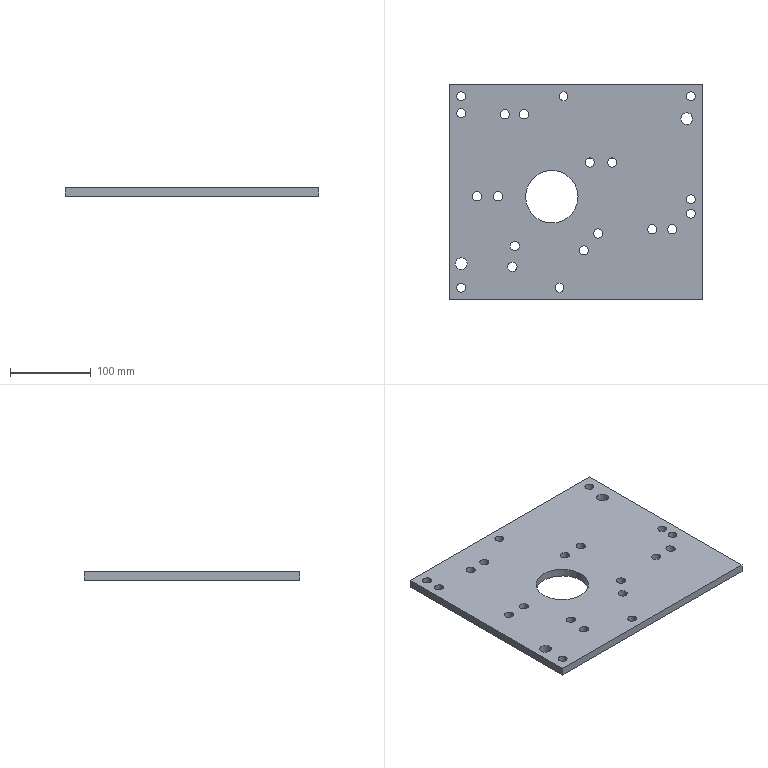Part | STEP file | lll_id3002_x_t | 1 solid | 29 faces | box 315 x 268 x 10 mm | volume 787421 mm3 | cylinder 23 | plane 6 | commonest cylinder face diameters 11.509 x12 11 x8 14.505 x2 65.2 x1
STEP:
#1=CARTESIAN_POINT('',(3328.121,63.788,92.5));
#2=VERTEX_POINT('',#1);
#3=CARTESIAN_POINT('',(3322.367,63.788,92.5));
#4=DIRECTION('',(0.,0.,1.));
#5=DIRECTION('',(1.,0.,0.));
#6=AXIS2_PLACEMENT_3D('',#3,#4,#5);
#7=CIRCLE('',#6,5.755);
#8=EDGE_CURVE('',#2,#2,#7,.T.);
#9=ORIENTED_EDGE('',*,*,#8,.F.);
#10=EDGE_LOOP('',(#9));
#11=FACE_BOUND('',#10,.T.);
#12=CARTESIAN_POINT('',(3316.612,63.788,102.5));
#13=VERTEX_POINT('',#12);
#14=CARTESIAN_POINT('',(3322.367,63.788,102.5));
#15=DIRECTION('',(0.,0.,-1.));
#16=DIRECTION('',(-1.,0.,0.));
#17=AXIS2_PLACEMENT_3D('',#14,#15,#16);
#18=CIRCLE('',#17,5.755);
#19=EDGE_CURVE('',#13,#13,#18,.T.);
#20=ORIENTED_EDGE('',*,*,#19,.F.);
#21=EDGE_LOOP('',(#20));
#22=FACE_BOUND('',#21,.T.);
#23=CARTESIAN_POINT('',(3322.367,63.788,79.5));
#24=DIRECTION('',(0.,0.,1.));
#25=DIRECTION('',(1.,0.,0.));
#26=AXIS2_PLACEMENT_3D('',#23,#24,#25);
#27=CYLINDRICAL_SURFACE('',#26,5.755);
#28=ADVANCED_FACE('',(#11,#22),#27,.F.);
#29=CARTESIAN_POINT('',(3449.867,127.288,102.5));
#30=VERTEX_POINT('',#29);
#31=CARTESIAN_POINT('',(3455.367,127.288,102.5));
#32=DIRECTION('',(0.,0.,1.));
#33=DIRECTION('',(-1.,0.,0.));
#34=AXIS2_PLACEMENT_3D('',#31,#32,#33);
#35=CIRCLE('',#34,5.5);
#36=EDGE_CURVE('',#30,#30,#35,.T.);
#37=ORIENTED_EDGE('',*,*,#36,.T.);
#38=EDGE_LOOP('',(#37));
#39=FACE_BOUND('',#38,.T.);
#40=CARTESIAN_POINT('',(3460.867,127.288,92.5));
#41=VERTEX_POINT('',#40);
#42=CARTESIAN_POINT('',(3455.367,127.288,92.5));
#43=DIRECTION('',(0.,0.,-1.));
#44=DIRECTION('',(1.,0.,0.));
#45=AXIS2_PLACEMENT_3D('',#42,#43,#44);
#46=CIRCLE('',#45,5.5);
#47=EDGE_CURVE('',#41,#41,#46,.T.);
#48=ORIENTED_EDGE('',*,*,#47,.T.);
#49=EDGE_LOOP('',(#48));
#50=FACE_BOUND('',#49,.T.);
#51=CARTESIAN_POINT('',(3455.367,127.288,92.5));
#52=DIRECTION('',(0.,0.,1.));
#53=DIRECTION('',(-1.,0.,0.));
#54=AXIS2_PLACEMENT_3D('',#51,#52,#53);
#55=CYLINDRICAL_SURFACE('',#54,5.5);
#56=ADVANCED_FACE('',(#39,#50),#55,.F.);
#57=CARTESIAN_POINT('',(3449.867,109.288,102.5));
#58=VERTEX_POINT('',#57);
#59=CARTESIAN_POINT('',(3455.367,109.288,102.5));
#60=DIRECTION('',(0.,0.,1.));
#61=DIRECTION('',(-1.,0.,0.));
#62=AXIS2_PLACEMENT_3D('',#59,#60,#61);
#63=CIRCLE('',#62,5.5);
#64=EDGE_CURVE('',#58,#58,#63,.T.);
#65=ORIENTED_EDGE('',*,*,#64,.T.);
#66=EDGE_LOOP('',(#65));
#67=FACE_BOUND('',#66,.T.);
#68=CARTESIAN_POINT('',(3449.867,109.288,92.5));
#69=VERTEX_POINT('',#68);
#70=CARTESIAN_POINT('',(3455.367,109.288,92.5));
#71=DIRECTION('',(0.,0.,-1.));
#72=DIRECTION('',(-1.,0.,0.));
#73=AXIS2_PLACEMENT_3D('',#70,#71,#72);
#74=CIRCLE('',#73,5.5);
#75=EDGE_CURVE('',#69,#69,#74,.T.);
#76=ORIENTED_EDGE('',*,*,#75,.T.);
#77=EDGE_LOOP('',(#76));
#78=FACE_BOUND('',#77,.T.);
#79=CARTESIAN_POINT('',(3455.367,109.288,92.5));
#80=DIRECTION('',(0.,0.,1.));
#81=DIRECTION('',(-1.,0.,0.));
#82=AXIS2_PLACEMENT_3D('',#79,#80,#81);
#83=CYLINDRICAL_SURFACE('',#82,5.5);
#84=ADVANCED_FACE('',(#67,#78),#83,.F.);
#85=CARTESIAN_POINT('',(3155.367,270.288,102.5));
#86=VERTEX_POINT('',#85);
#87=CARTESIAN_POINT('',(3155.367,270.288,92.5));
#88=VERTEX_POINT('',#87);
#89=CARTESIAN_POINT('',(3155.367,270.288,92.5));
#90=DIRECTION('',(0.,0.,-1.));
#91=VECTOR('',#90,1.);
#92=LINE('',#89,#91);
#93=EDGE_CURVE('',#86,#88,#92,.T.);
#94=ORIENTED_EDGE('',*,*,#93,.F.);
#95=CARTESIAN_POINT('',(3470.367,270.288,102.5));
#96=VERTEX_POINT('',#95);
#97=CARTESIAN_POINT('',(3227.867,270.288,102.5));
#98=DIRECTION('',(-1.,0.,0.));
#99=VECTOR('',#98,1.);
#100=LINE('',#97,#99);
#101=EDGE_CURVE('',#96,#86,#100,.T.);
#102=ORIENTED_EDGE('',*,*,#101,.F.);
#103=CARTESIAN_POINT('',(3470.367,270.288,92.5));
#104=VERTEX_POINT('',#103);
#105=CARTESIAN_POINT('',(3470.367,270.288,92.5));
#106=DIRECTION('',(0.,0.,-1.));
#107=VECTOR('',#106,1.);
#108=LINE('',#105,#107);
#109=EDGE_CURVE('',#96,#104,#108,.T.);
#110=ORIENTED_EDGE('',*,*,#109,.T.);
#111=CARTESIAN_POINT('',(3227.867,270.288,92.5));
#112=DIRECTION('',(-1.,0.,0.));
#113=VECTOR('',#112,1.);
#114=LINE('',#111,#113);
#115=EDGE_CURVE('',#104,#88,#114,.T.);
#116=ORIENTED_EDGE('',*,*,#115,.T.);
#117=EDGE_LOOP('',(#94,#102,#110,#116));
#118=FACE_OUTER_BOUND('',#117,.T.);
#119=CARTESIAN_POINT('',(3227.867,270.288,92.5));
#120=DIRECTION('',(0.,1.,0.));
#121=DIRECTION('',(-1.,0.,0.));
#122=AXIS2_PLACEMENT_3D('',#119,#120,#121);
#123=PLANE('',#122);
#124=ADVANCED_FACE('',(#118),#123,.T.);
#125=ORIENTED_EDGE('',*,*,#109,.F.);
#126=CARTESIAN_POINT('',(3470.367,2.288,102.5));
#127=VERTEX_POINT('',#126);
#128=CARTESIAN_POINT('',(3470.367,195.288,102.5));
#129=DIRECTION('',(0.,1.,0.));
#130=VECTOR('',#129,1.);
#131=LINE('',#128,#130);
#132=EDGE_CURVE('',#127,#96,#131,.T.);
#133=ORIENTED_EDGE('',*,*,#132,.F.);
#134=CARTESIAN_POINT('',(3470.367,2.288,92.5));
#135=VERTEX_POINT('',#134);
#136=CARTESIAN_POINT('',(3470.367,2.288,92.5));
#137=DIRECTION('',(0.,0.,-1.));
#138=VECTOR('',#137,1.);
#139=LINE('',#136,#138);
#140=EDGE_CURVE('',#127,#135,#139,.T.);
#141=ORIENTED_EDGE('',*,*,#140,.T.);
#142=CARTESIAN_POINT('',(3470.367,195.288,92.5));
#143=DIRECTION('',(0.,1.,0.));
#144=VECTOR('',#143,1.);
#145=LINE('',#142,#144);
#146=EDGE_CURVE('',#135,#104,#145,.T.);
#147=ORIENTED_EDGE('',*,*,#146,.T.);
#148=EDGE_LOOP('',(#125,#133,#141,#147));
#149=FACE_OUTER_BOUND('',#148,.T.);
#150=CARTESIAN_POINT('',(3470.367,195.288,92.5));
#151=DIRECTION('',(1.,0.,0.));
#152=DIRECTION('',(0.,1.,0.));
#153=AXIS2_PLACEMENT_3D('',#150,#151,#152);
#154=PLANE('',#153);
#155=ADVANCED_FACE('',(#149),#154,.T.);
#156=ORIENTED_EDGE('',*,*,#140,.F.);
#157=CARTESIAN_POINT('',(3155.367,2.288,102.5));
#158=VERTEX_POINT('',#157);
#159=CARTESIAN_POINT('',(3227.867,2.288,102.5));
#160=DIRECTION('',(-1.,0.,0.));
#161=VECTOR('',#160,1.);
#162=LINE('',#159,#161);
#163=EDGE_CURVE('',#127,#158,#162,.T.);
#164=ORIENTED_EDGE('',*,*,#163,.T.);
#165=CARTESIAN_POINT('',(3155.367,2.288,92.5));
#166=VERTEX_POINT('',#165);
#167=CARTESIAN_POINT('',(3155.367,2.288,92.5));
#168=DIRECTION('',(0.,0.,-1.));
#169=VECTOR('',#168,1.);
#170=LINE('',#167,#169);
#171=EDGE_CURVE('',#158,#166,#170,.T.);
#172=ORIENTED_EDGE('',*,*,#171,.T.);
#173=CARTESIAN_POINT('',(3227.867,2.288,92.5));
#174=DIRECTION('',(1.,0.,0.));
#175=VECTOR('',#174,1.);
#176=LINE('',#173,#175);
#177=EDGE_CURVE('',#166,#135,#176,.T.);
#178=ORIENTED_EDGE('',*,*,#177,.T.);
#179=EDGE_LOOP('',(#156,#164,#172,#178));
#180=FACE_OUTER_BOUND('',#179,.T.);
#181=CARTESIAN_POINT('',(3227.867,2.288,92.5));
#182=DIRECTION('',(0.,-1.,0.));
#183=DIRECTION('',(1.,0.,0.));
#184=AXIS2_PLACEMENT_3D('',#181,#182,#183);
#185=PLANE('',#184);
#186=ADVANCED_FACE('',(#180),#185,.T.);
#187=ORIENTED_EDGE('',*,*,#171,.F.);
#188=CARTESIAN_POINT('',(3155.367,166.13,102.5));
#189=DIRECTION('',(0.,1.,0.));
#190=VECTOR('',#189,1.);
#191=LINE('',#188,#190);
#192=EDGE_CURVE('',#158,#86,#191,.T.);
#193=ORIENTED_EDGE('',*,*,#192,.T.);
#194=ORIENTED_EDGE('',*,*,#93,.T.);
#195=CARTESIAN_POINT('',(3155.367,166.13,92.5));
#196=DIRECTION('',(0.,1.,0.));
#197=VECTOR('',#196,1.);
#198=LINE('',#195,#197);
#199=EDGE_CURVE('',#166,#88,#198,.T.);
#200=ORIENTED_EDGE('',*,*,#199,.F.);
#201=EDGE_LOOP('',(#187,#193,#194,#200));
#202=FACE_OUTER_BOUND('',#201,.T.);
#203=CARTESIAN_POINT('',(3155.367,166.13,92.5));
#204=DIRECTION('',(1.,0.,0.));
#205=DIRECTION('',(0.,1.,0.));
#206=AXIS2_PLACEMENT_3D('',#203,#204,#205);
#207=PLANE('',#206);
#208=ADVANCED_FACE('',(#202),#207,.F.);
#209=CARTESIAN_POINT('',(3449.867,255.288,102.5));
#210=VERTEX_POINT('',#209);
#211=CARTESIAN_POINT('',(3455.367,255.288,102.5));
#212=DIRECTION('',(0.,0.,1.));
#213=DIRECTION('',(-1.,0.,0.));
#214=AXIS2_PLACEMENT_3D('',#211,#212,#213);
#215=CIRCLE('',#214,5.5);
#216=EDGE_CURVE('',#210,#210,#215,.T.);
#217=ORIENTED_EDGE('',*,*,#216,.T.);
#218=EDGE_LOOP('',(#217));
#219=FACE_BOUND('',#218,.T.);
#220=CARTESIAN_POINT('',(3449.867,255.288,92.5));
#221=VERTEX_POINT('',#220);
#222=CARTESIAN_POINT('',(3455.367,255.288,92.5));
#223=DIRECTION('',(0.,0.,1.));
#224=DIRECTION('',(-1.,0.,0.));
#225=AXIS2_PLACEMENT_3D('',#222,#223,#224);
#226=CIRCLE('',#225,5.5);
#227=EDGE_CURVE('',#221,#221,#226,.T.);
#228=ORIENTED_EDGE('',*,*,#227,.F.);
#229=EDGE_LOOP('',(#228));
#230=FACE_BOUND('',#229,.T.);
#231=CARTESIAN_POINT('',(3455.367,255.288,92.5));
#232=DIRECTION('',(0.,0.,1.));
#233=DIRECTION('',(-1.,0.,0.));
#234=AXIS2_PLACEMENT_3D('',#231,#232,#233);
#235=CYLINDRICAL_SURFACE('',#234,5.5);
#236=ADVANCED_FACE('',(#219,#230),#235,.F.);
#237=CARTESIAN_POINT('',(3286.867,17.288,102.5));
#238=VERTEX_POINT('',#237);
#239=CARTESIAN_POINT('',(3292.367,17.288,102.5));
#240=DIRECTION('',(0.,0.,-1.));
#241=DIRECTION('',(-1.,0.,0.));
#242=AXIS2_PLACEMENT_3D('',#239,#240,#241);
#243=CIRCLE('',#242,5.5);
#244=EDGE_CURVE('',#238,#238,#243,.T.);
#245=ORIENTED_EDGE('',*,*,#244,.F.);
#246=EDGE_LOOP('',(#245));
#247=FACE_BOUND('',#246,.T.);
#248=CARTESIAN_POINT('',(3286.867,17.288,92.5));
#249=VERTEX_POINT('',#248);
#250=CARTESIAN_POINT('',(3292.367,17.288,92.5));
#251=DIRECTION('',(0.,0.,1.));
#252=DIRECTION('',(-1.,0.,0.));
#253=AXIS2_PLACEMENT_3D('',#250,#251,#252);
#254=CIRCLE('',#253,5.5);
#255=EDGE_CURVE('',#249,#249,#254,.T.);
#256=ORIENTED_EDGE('',*,*,#255,.F.);
#257=EDGE_LOOP('',(#256));
#258=FACE_BOUND('',#257,.T.);
#259=CARTESIAN_POINT('',(3292.367,17.288,92.5));
#260=DIRECTION('',(0.,0.,1.));
#261=DIRECTION('',(-1.,0.,0.));
#262=AXIS2_PLACEMENT_3D('',#259,#260,#261);
#263=CYLINDRICAL_SURFACE('',#262,5.5);
#264=ADVANCED_FACE('',(#247,#258),#263,.F.);
#265=CARTESIAN_POINT('',(3163.115,47.288,102.5));
#266=VERTEX_POINT('',#265);
#267=CARTESIAN_POINT('',(3170.367,47.288,102.5));
#268=DIRECTION('',(0.,0.,-1.));
#269=DIRECTION('',(-1.,0.,0.));
#270=AXIS2_PLACEMENT_3D('',#267,#268,#269);
#271=CIRCLE('',#270,7.253);
#272=EDGE_CURVE('',#266,#266,#271,.T.);
#273=ORIENTED_EDGE('',*,*,#272,.F.);
#274=EDGE_LOOP('',(#273));
#275=FACE_BOUND('',#274,.T.);
#276=CARTESIAN_POINT('',(3177.62,47.288,92.5));
#277=VERTEX_POINT('',#276);
#278=CARTESIAN_POINT('',(3170.367,47.288,92.5));
#279=DIRECTION('',(0.,0.,1.));
#280=DIRECTION('',(1.,0.,0.));
#281=AXIS2_PLACEMENT_3D('',#278,#279,#280);
#282=CIRCLE('',#281,7.253);
#283=EDGE_CURVE('',#277,#277,#282,.T.);
#284=ORIENTED_EDGE('',*,*,#283,.F.);
#285=EDGE_LOOP('',(#284));
#286=FACE_BOUND('',#285,.T.);
#287=CARTESIAN_POINT('',(3170.367,47.288,92.5));
#288=DIRECTION('',(0.,0.,1.));
#289=DIRECTION('',(1.,0.,0.));
#290=AXIS2_PLACEMENT_3D('',#287,#288,#289);
#291=CYLINDRICAL_SURFACE('',#290,7.253);
#292=ADVANCED_FACE('',(#275,#286),#291,.F.);
#293=CARTESIAN_POINT('',(3443.115,227.288,102.5));
#294=VERTEX_POINT('',#293);
#295=CARTESIAN_POINT('',(3450.367,227.288,102.5));
#296=DIRECTION('',(0.,0.,-1.));
#297=DIRECTION('',(-1.,0.,0.));
#298=AXIS2_PLACEMENT_3D('',#295,#296,#297);
#299=CIRCLE('',#298,7.253);
#300=EDGE_CURVE('',#294,#294,#299,.T.);
#301=ORIENTED_EDGE('',*,*,#300,.F.);
#302=EDGE_LOOP('',(#301));
#303=FACE_BOUND('',#302,.T.);
#304=CARTESIAN_POINT('',(3457.62,227.288,92.5));
#305=VERTEX_POINT('',#304);
#306=CARTESIAN_POINT('',(3450.367,227.288,92.5));
#307=DIRECTION('',(0.,0.,1.));
#308=DIRECTION('',(1.,0.,0.));
#309=AXIS2_PLACEMENT_3D('',#306,#307,#308);
#310=CIRCLE('',#309,7.253);
#311=EDGE_CURVE('',#305,#305,#310,.T.);
#312=ORIENTED_EDGE('',*,*,#311,.F.);
#313=EDGE_LOOP('',(#312));
#314=FACE_BOUND('',#313,.T.);
#315=CARTESIAN_POINT('',(3450.367,227.288,92.5));
#316=DIRECTION('',(0.,0.,1.));
#317=DIRECTION('',(1.,0.,0.));
#318=AXIS2_PLACEMENT_3D('',#315,#316,#317);
#319=CYLINDRICAL_SURFACE('',#318,7.253);
#320=ADVANCED_FACE('',(#303,#314),#319,.F.);
#321=CARTESIAN_POINT('',(3291.867,255.288,102.5));
#322=VERTEX_POINT('',#321);
#323=CARTESIAN_POINT('',(3297.367,255.288,102.5));
#324=DIRECTION('',(0.,0.,1.));
#325=DIRECTION('',(-1.,0.,0.));
#326=AXIS2_PLACEMENT_3D('',#323,#324,#325);
#327=CIRCLE('',#326,5.5);
#328=EDGE_CURVE('',#322,#322,#327,.T.);
#329=ORIENTED_EDGE('',*,*,#328,.T.);
#330=EDGE_LOOP('',(#329));
#331=FACE_BOUND('',#330,.T.);
#332=CARTESIAN_POINT('',(3291.867,255.288,92.5));
#333=VERTEX_POINT('',#332);
#334=CARTESIAN_POINT('',(3297.367,255.288,92.5));
#335=DIRECTION('',(0.,0.,1.));
#336=DIRECTION('',(-1.,0.,0.));
#337=AXIS2_PLACEMENT_3D('',#334,#335,#336);
#338=CIRCLE('',#337,5.5);
#339=EDGE_CURVE('',#333,#333,#338,.T.);
#340=ORIENTED_EDGE('',*,*,#339,.F.);
#341=EDGE_LOOP('',(#340));
#342=FACE_BOUND('',#341,.T.);
#343=CARTESIAN_POINT('',(3297.367,255.288,92.5));
#344=DIRECTION('',(0.,0.,1.));
#345=DIRECTION('',(-1.,0.,0.));
#346=AXIS2_PLACEMENT_3D('',#343,#344,#345);
#347=CYLINDRICAL_SURFACE('',#346,5.5);
#348=ADVANCED_FACE('',(#331,#342),#347,.F.);
#349=CARTESIAN_POINT('',(3164.867,255.288,102.5));
#350=VERTEX_POINT('',#349);
#351=CARTESIAN_POINT('',(3170.367,255.288,102.5));
#352=DIRECTION('',(0.,0.,1.));
#353=DIRECTION('',(-1.,0.,0.));
#354=AXIS2_PLACEMENT_3D('',#351,#352,#353);
#355=CIRCLE('',#354,5.5);
#356=EDGE_CURVE('',#350,#350,#355,.T.);
#357=ORIENTED_EDGE('',*,*,#356,.T.);
#358=EDGE_LOOP('',(#357));
#359=FACE_BOUND('',#358,.T.);
#360=CARTESIAN_POINT('',(3164.867,255.288,92.5));
#361=VERTEX_POINT('',#360);
#362=CARTESIAN_POINT('',(3170.367,255.288,92.5));
#363=DIRECTION('',(0.,0.,-1.));
#364=DIRECTION('',(-1.,0.,0.));
#365=AXIS2_PLACEMENT_3D('',#362,#363,#364);
#366=CIRCLE('',#365,5.5);
#367=EDGE_CURVE('',#361,#361,#366,.T.);
#368=ORIENTED_EDGE('',*,*,#367,.T.);
#369=EDGE_LOOP('',(#368));
#370=FACE_BOUND('',#369,.T.);
#371=CARTESIAN_POINT('',(3170.367,255.288,92.5));
#372=DIRECTION('',(0.,0.,1.));
#373=DIRECTION('',(-1.,0.,0.));
#374=AXIS2_PLACEMENT_3D('',#371,#372,#373);
#375=CYLINDRICAL_SURFACE('',#374,5.5);
#376=ADVANCED_FACE('',(#359,#370),#375,.F.);
#377=CARTESIAN_POINT('',(3164.867,17.288,102.5));
#378=VERTEX_POINT('',#377);
#379=CARTESIAN_POINT('',(3170.367,17.288,102.5));
#380=DIRECTION('',(0.,0.,-1.));
#381=DIRECTION('',(-1.,0.,0.));
#382=AXIS2_PLACEMENT_3D('',#379,#380,#381);
#383=CIRCLE('',#382,5.5);
#384=EDGE_CURVE('',#378,#378,#383,.T.);
#385=ORIENTED_EDGE('',*,*,#384,.F.);
#386=EDGE_LOOP('',(#385));
#387=FACE_BOUND('',#386,.T.);
#388=CARTESIAN_POINT('',(3164.867,17.288,92.5));
#389=VERTEX_POINT('',#388);
#390=CARTESIAN_POINT('',(3170.367,17.288,92.5));
#391=DIRECTION('',(0.,0.,-1.));
#392=DIRECTION('',(-1.,0.,0.));
#393=AXIS2_PLACEMENT_3D('',#390,#391,#392);
#394=CIRCLE('',#393,5.5);
#395=EDGE_CURVE('',#389,#389,#394,.T.);
#396=ORIENTED_EDGE('',*,*,#395,.T.);
#397=EDGE_LOOP('',(#396));
#398=FACE_BOUND('',#397,.T.);
#399=CARTESIAN_POINT('',(3170.367,17.288,92.5));
#400=DIRECTION('',(0.,0.,1.));
#401=DIRECTION('',(-1.,0.,0.));
#402=AXIS2_PLACEMENT_3D('',#399,#400,#401);
#403=CYLINDRICAL_SURFACE('',#402,5.5);
#404=ADVANCED_FACE('',(#387,#398),#403,.F.);
#405=CARTESIAN_POINT('',(3164.867,234.288,102.5));
#406=VERTEX_POINT('',#405);
#407=CARTESIAN_POINT('',(3170.367,234.288,102.5));
#408=DIRECTION('',(0.,0.,1.));
#409=DIRECTION('',(-1.,0.,0.));
#410=AXIS2_PLACEMENT_3D('',#407,#408,#409);
#411=CIRCLE('',#410,5.5);
#412=EDGE_CURVE('',#406,#406,#411,.T.);
#413=ORIENTED_EDGE('',*,*,#412,.T.);
#414=EDGE_LOOP('',(#413));
#415=FACE_BOUND('',#414,.T.);
#416=CARTESIAN_POINT('',(3175.867,234.288,92.5));
#417=VERTEX_POINT('',#416);
#418=CARTESIAN_POINT('',(3170.367,234.288,92.5));
#419=DIRECTION('',(0.,0.,-1.));
#420=DIRECTION('',(1.,0.,0.));
#421=AXIS2_PLACEMENT_3D('',#418,#419,#420);
#422=CIRCLE('',#421,5.5);
#423=EDGE_CURVE('',#417,#417,#422,.T.);
#424=ORIENTED_EDGE('',*,*,#423,.T.);
#425=EDGE_LOOP('',(#424));
#426=FACE_BOUND('',#425,.T.);
#427=CARTESIAN_POINT('',(3170.367,234.288,92.5));
#428=DIRECTION('',(0.,0.,1.));
#429=DIRECTION('',(-1.,0.,0.));
#430=AXIS2_PLACEMENT_3D('',#427,#428,#429);
#431=CYLINDRICAL_SURFACE('',#430,5.5);
#432=ADVANCED_FACE('',(#415,#426),#431,.F.);
#433=CARTESIAN_POINT('',(3221.755,131.,92.5));
#434=VERTEX_POINT('',#433);
#435=CARTESIAN_POINT('',(3216.,131.,92.5));
#436=DIRECTION('',(0.,0.,-1.));
#437=DIRECTION('',(1.,0.,0.));
#438=AXIS2_PLACEMENT_3D('',#435,#436,#437);
#439=CIRCLE('',#438,5.755);
#440=EDGE_CURVE('',#434,#434,#439,.T.);
#441=ORIENTED_EDGE('',*,*,#440,.T.);
#442=EDGE_LOOP('',(#441));
#443=FACE_BOUND('',#442,.T.);
#444=CARTESIAN_POINT('',(3210.246,131.,102.5));
#445=VERTEX_POINT('',#444);
#446=CARTESIAN_POINT('',(3216.,131.,102.5));
#447=DIRECTION('',(0.,0.,-1.));
#448=DIRECTION('',(-1.,0.,0.));
#449=AXIS2_PLACEMENT_3D('',#446,#447,#448);
#450=CIRCLE('',#449,5.755);
#451=EDGE_CURVE('',#445,#445,#450,.T.);
#452=ORIENTED_EDGE('',*,*,#451,.F.);
#453=EDGE_LOOP('',(#452));
#454=FACE_BOUND('',#453,.T.);
#455=CARTESIAN_POINT('',(3216.,131.,79.5));
#456=DIRECTION('',(0.,0.,1.));
#457=DIRECTION('',(1.,0.,0.));
#458=AXIS2_PLACEMENT_3D('',#455,#456,#457);
#459=CYLINDRICAL_SURFACE('',#458,5.755);
#460=ADVANCED_FACE('',(#443,#454),#459,.F.);
#461=CARTESIAN_POINT('',(3363.622,172.788,92.5));
#462=VERTEX_POINT('',#461);
#463=CARTESIAN_POINT('',(3357.867,172.788,92.5));
#464=DIRECTION('',(0.,0.,-1.));
#465=DIRECTION('',(1.,0.,0.));
#466=AXIS2_PLACEMENT_3D('',#463,#464,#465);
#467=CIRCLE('',#466,5.755);
#468=EDGE_CURVE('',#462,#462,#467,.T.);
#469=ORIENTED_EDGE('',*,*,#468,.T.);
#470=EDGE_LOOP('',(#469));
#471=FACE_BOUND('',#470,.T.);
#472=CARTESIAN_POINT('',(3352.113,172.788,102.5));
#473=VERTEX_POINT('',#472);
#474=CARTESIAN_POINT('',(3357.867,172.788,102.5));
#475=DIRECTION('',(0.,0.,-1.));
#476=DIRECTION('',(-1.,0.,0.));
#477=AXIS2_PLACEMENT_3D('',#474,#475,#476);
#478=CIRCLE('',#477,5.755);
#479=EDGE_CURVE('',#473,#473,#478,.T.);
#480=ORIENTED_EDGE('',*,*,#479,.F.);
#481=EDGE_LOOP('',(#480));
#482=FACE_BOUND('',#481,.T.);
#483=CARTESIAN_POINT('',(3357.867,172.788,79.5));
#484=DIRECTION('',(0.,0.,1.));
#485=DIRECTION('',(1.,0.,0.));
#486=AXIS2_PLACEMENT_3D('',#483,#484,#485);
#487=CYLINDRICAL_SURFACE('',#486,5.755);
#488=ADVANCED_FACE('',(#471,#482),#487,.F.);
#489=CARTESIAN_POINT('',(3242.731,69.288,92.5));
#490=VERTEX_POINT('',#489);
#491=CARTESIAN_POINT('',(3236.977,69.288,92.5));
#492=DIRECTION('',(0.,0.,-1.));
#493=DIRECTION('',(1.,0.,0.));
#494=AXIS2_PLACEMENT_3D('',#491,#492,#493);
#495=CIRCLE('',#494,5.755);
#496=EDGE_CURVE('',#490,#490,#495,.T.);
#497=ORIENTED_EDGE('',*,*,#496,.T.);
#498=EDGE_LOOP('',(#497));
#499=FACE_BOUND('',#498,.T.);
#500=CARTESIAN_POINT('',(3231.222,69.288,102.5));
#501=VERTEX_POINT('',#500);
#502=CARTESIAN_POINT('',(3236.977,69.288,102.5));
#503=DIRECTION('',(0.,0.,-1.));
#504=DIRECTION('',(-1.,0.,0.));
#505=AXIS2_PLACEMENT_3D('',#502,#503,#504);
#506=CIRCLE('',#505,5.755);
#507=EDGE_CURVE('',#501,#501,#506,.T.);
#508=ORIENTED_EDGE('',*,*,#507,.F.);
#509=EDGE_LOOP('',(#508));
#510=FACE_BOUND('',#509,.T.);
#511=CARTESIAN_POINT('',(3236.977,69.288,79.5));
#512=DIRECTION('',(0.,0.,1.));
#513=DIRECTION('',(1.,0.,0.));
#514=AXIS2_PLACEMENT_3D('',#511,#512,#513);
#515=CYLINDRICAL_SURFACE('',#514,5.755);
#516=ADVANCED_FACE('',(#499,#510),#515,.F.);
#517=CARTESIAN_POINT('',(3346.121,84.788,92.5));
#518=VERTEX_POINT('',#517);
#519=CARTESIAN_POINT('',(3340.367,84.788,92.5));
#520=DIRECTION('',(0.,0.,-1.));
#521=DIRECTION('',(1.,0.,0.));
#522=AXIS2_PLACEMENT_3D('',#519,#520,#521);
#523=CIRCLE('',#522,5.755);
#524=EDGE_CURVE('',#518,#518,#523,.T.);
#525=ORIENTED_EDGE('',*,*,#524,.T.);
#526=EDGE_LOOP('',(#525));
#527=FACE_BOUND('',#526,.T.);
#528=CARTESIAN_POINT('',(3334.612,84.788,102.5));
#529=VERTEX_POINT('',#528);
#530=CARTESIAN_POINT('',(3340.367,84.788,102.5));
#531=DIRECTION('',(0.,0.,-1.));
#532=DIRECTION('',(-1.,0.,0.));
#533=AXIS2_PLACEMENT_3D('',#530,#531,#532);
#534=CIRCLE('',#533,5.755);
#535=EDGE_CURVE('',#529,#529,#534,.T.);
#536=ORIENTED_EDGE('',*,*,#535,.F.);
#537=EDGE_LOOP('',(#536));
#538=FACE_BOUND('',#537,.T.);
#539=CARTESIAN_POINT('',(3340.367,84.788,79.5));
#540=DIRECTION('',(0.,0.,1.));
#541=DIRECTION('',(1.,0.,0.));
#542=AXIS2_PLACEMENT_3D('',#539,#540,#541);
#543=CYLINDRICAL_SURFACE('',#542,5.755);
#544=ADVANCED_FACE('',(#527,#538),#543,.F.);
#545=CARTESIAN_POINT('',(3413.255,90.,92.5));
#546=VERTEX_POINT('',#545);
#547=CARTESIAN_POINT('',(3407.5,90.,92.5));
#548=DIRECTION('',(0.,0.,-1.));
#549=DIRECTION('',(1.,0.,0.));
#550=AXIS2_PLACEMENT_3D('',#547,#548,#549);
#551=CIRCLE('',#550,5.755);
#552=EDGE_CURVE('',#546,#546,#551,.T.);
#553=ORIENTED_EDGE('',*,*,#552,.T.);
#554=EDGE_LOOP('',(#553));
#555=FACE_BOUND('',#554,.T.);
#556=CARTESIAN_POINT('',(3401.746,90.,102.5));
#557=VERTEX_POINT('',#556);
#558=CARTESIAN_POINT('',(3407.5,90.,102.5));
#559=DIRECTION('',(0.,0.,-1.));
#560=DIRECTION('',(-1.,0.,0.));
#561=AXIS2_PLACEMENT_3D('',#558,#559,#560);
#562=CIRCLE('',#561,5.755);
#563=EDGE_CURVE('',#557,#557,#562,.T.);
#564=ORIENTED_EDGE('',*,*,#563,.F.);
#565=EDGE_LOOP('',(#564));
#566=FACE_BOUND('',#565,.T.);
#567=CARTESIAN_POINT('',(3407.5,90.,79.5));
#568=DIRECTION('',(0.,0.,1.));
#569=DIRECTION('',(1.,0.,0.));
#570=AXIS2_PLACEMENT_3D('',#567,#568,#569);
#571=CYLINDRICAL_SURFACE('',#570,5.755);
#572=ADVANCED_FACE('',(#555,#566),#571,.F.);
#573=CARTESIAN_POINT('',(3250.256,130.4,102.5));
#574=VERTEX_POINT('',#573);
#575=CARTESIAN_POINT('',(3282.856,130.4,102.5));
#576=DIRECTION('',(0.,0.,-1.));
#577=DIRECTION('',(-1.,0.,0.));
#578=AXIS2_PLACEMENT_3D('',#575,#576,#577);
#579=CIRCLE('',#578,32.6);
#580=EDGE_CURVE('',#574,#574,#579,.T.);
#581=ORIENTED_EDGE('',*,*,#580,.F.);
#582=EDGE_LOOP('',(#581));
#583=FACE_BOUND('',#582,.T.);
#584=CARTESIAN_POINT('',(3315.456,130.4,92.5));
#585=VERTEX_POINT('',#584);
#586=CARTESIAN_POINT('',(3282.856,130.4,92.5));
#587=DIRECTION('',(0.,0.,1.));
#588=DIRECTION('',(1.,0.,0.));
#589=AXIS2_PLACEMENT_3D('',#586,#587,#588);
#590=CIRCLE('',#589,32.6);
#591=EDGE_CURVE('',#585,#585,#590,.T.);
#592=ORIENTED_EDGE('',*,*,#591,.F.);
#593=EDGE_LOOP('',(#592));
#594=FACE_BOUND('',#593,.T.);
#595=CARTESIAN_POINT('',(3282.856,130.4,-257.5));
#596=DIRECTION('',(0.,0.,1.));
#597=DIRECTION('',(1.,0.,0.));
#598=AXIS2_PLACEMENT_3D('',#595,#596,#597);
#599=CYLINDRICAL_SURFACE('',#598,32.6);
#600=ADVANCED_FACE('',(#583,#594),#599,.F.);
#601=CARTESIAN_POINT('',(3254.121,232.788,92.5));
#602=VERTEX_POINT('',#601);
#603=CARTESIAN_POINT('',(3248.367,232.788,92.5));
#604=DIRECTION('',(0.,0.,1.));
#605=DIRECTION('',(1.,0.,0.));
#606=AXIS2_PLACEMENT_3D('',#603,#604,#605);
#607=CIRCLE('',#606,5.755);
#608=EDGE_CURVE('',#602,#602,#607,.T.);
#609=ORIENTED_EDGE('',*,*,#608,.F.);
#610=EDGE_LOOP('',(#609));
#611=FACE_BOUND('',#610,.T.);
#612=CARTESIAN_POINT('',(3242.612,232.788,102.5));
#613=VERTEX_POINT('',#612);
#614=CARTESIAN_POINT('',(3248.367,232.788,102.5));
#615=DIRECTION('',(0.,0.,-1.));
#616=DIRECTION('',(-1.,0.,0.));
#617=AXIS2_PLACEMENT_3D('',#614,#615,#616);
#618=CIRCLE('',#617,5.755);
#619=EDGE_CURVE('',#613,#613,#618,.T.);
#620=ORIENTED_EDGE('',*,*,#619,.F.);
#621=EDGE_LOOP('',(#620));
#622=FACE_BOUND('',#621,.T.);
#623=CARTESIAN_POINT('',(3248.367,232.788,79.5));
#624=DIRECTION('',(0.,0.,1.));
#625=DIRECTION('',(1.,0.,0.));
#626=AXIS2_PLACEMENT_3D('',#623,#624,#625);
#627=CYLINDRICAL_SURFACE('',#626,5.755);
#628=ADVANCED_FACE('',(#611,#622),#627,.F.);
#629=CARTESIAN_POINT('',(3230.121,232.788,92.5));
#630=VERTEX_POINT('',#629);
#631=CARTESIAN_POINT('',(3224.367,232.788,92.5));
#632=DIRECTION('',(0.,0.,1.));
#633=DIRECTION('',(1.,0.,0.));
#634=AXIS2_PLACEMENT_3D('',#631,#632,#633);
#635=CIRCLE('',#634,5.755);
#636=EDGE_CURVE('',#630,#630,#635,.T.);
#637=ORIENTED_EDGE('',*,*,#636,.F.);
#638=EDGE_LOOP('',(#637));
#639=FACE_BOUND('',#638,.T.);
#640=CARTESIAN_POINT('',(3218.612,232.788,102.5));
#641=VERTEX_POINT('',#640);
#642=CARTESIAN_POINT('',(3224.367,232.788,102.5));
#643=DIRECTION('',(0.,0.,-1.));
#644=DIRECTION('',(-1.,0.,0.));
#645=AXIS2_PLACEMENT_3D('',#642,#643,#644);
#646=CIRCLE('',#645,5.755);
#647=EDGE_CURVE('',#641,#641,#646,.T.);
#648=ORIENTED_EDGE('',*,*,#647,.F.);
#649=EDGE_LOOP('',(#648));
#650=FACE_BOUND('',#649,.T.);
#651=CARTESIAN_POINT('',(3224.367,232.788,79.5));
#652=DIRECTION('',(0.,0.,1.));
#653=DIRECTION('',(1.,0.,0.));
#654=AXIS2_PLACEMENT_3D('',#651,#652,#653);
#655=CYLINDRICAL_SURFACE('',#654,5.755);
#656=ADVANCED_FACE('',(#639,#650),#655,.F.);
#657=CARTESIAN_POINT('',(3335.622,172.788,92.5));
#658=VERTEX_POINT('',#657);
#659=CARTESIAN_POINT('',(3329.867,172.788,92.5));
#660=DIRECTION('',(0.,0.,1.));
#661=DIRECTION('',(1.,0.,0.));
#662=AXIS2_PLACEMENT_3D('',#659,#660,#661);
#663=CIRCLE('',#662,5.755);
#664=EDGE_CURVE('',#658,#658,#663,.T.);
#665=ORIENTED_EDGE('',*,*,#664,.F.);
#666=EDGE_LOOP('',(#665));
#667=FACE_BOUND('',#666,.T.);
#668=CARTESIAN_POINT('',(3324.113,172.788,102.5));
#669=VERTEX_POINT('',#668);
#670=CARTESIAN_POINT('',(3329.867,172.788,102.5));
#671=DIRECTION('',(0.,0.,-1.));
#672=DIRECTION('',(-1.,0.,0.));
#673=AXIS2_PLACEMENT_3D('',#670,#671,#672);
#674=CIRCLE('',#673,5.755);
#675=EDGE_CURVE('',#669,#669,#674,.T.);
#676=ORIENTED_EDGE('',*,*,#675,.F.);
#677=EDGE_LOOP('',(#676));
#678=FACE_BOUND('',#677,.T.);
#679=CARTESIAN_POINT('',(3329.867,172.788,79.5));
#680=DIRECTION('',(0.,0.,1.));
#681=DIRECTION('',(1.,0.,0.));
#682=AXIS2_PLACEMENT_3D('',#679,#680,#681);
#683=CYLINDRICAL_SURFACE('',#682,5.755);
#684=ADVANCED_FACE('',(#667,#678),#683,.F.);
#685=CARTESIAN_POINT('',(3438.254,90.,92.5));
#686=VERTEX_POINT('',#685);
#687=CARTESIAN_POINT('',(3432.5,90.,92.5));
#688=DIRECTION('',(0.,0.,1.));
#689=DIRECTION('',(1.,0.,0.));
#690=AXIS2_PLACEMENT_3D('',#687,#688,#689);
#691=CIRCLE('',#690,5.755);
#692=EDGE_CURVE('',#686,#686,#691,.T.);
#693=ORIENTED_EDGE('',*,*,#692,.F.);
#694=EDGE_LOOP('',(#693));
#695=FACE_BOUND('',#694,.T.);
#696=CARTESIAN_POINT('',(3426.745,90.,102.5));
#697=VERTEX_POINT('',#696);
#698=CARTESIAN_POINT('',(3432.5,90.,102.5));
#699=DIRECTION('',(0.,0.,-1.));
#700=DIRECTION('',(-1.,0.,0.));
#701=AXIS2_PLACEMENT_3D('',#698,#699,#700);
#702=CIRCLE('',#701,5.755);
#703=EDGE_CURVE('',#697,#697,#702,.T.);
#704=ORIENTED_EDGE('',*,*,#703,.F.);
#705=EDGE_LOOP('',(#704));
#706=FACE_BOUND('',#705,.T.);
#707=CARTESIAN_POINT('',(3432.5,90.,79.5));
#708=DIRECTION('',(0.,0.,1.));
#709=DIRECTION('',(1.,0.,0.));
#710=AXIS2_PLACEMENT_3D('',#707,#708,#709);
#711=CYLINDRICAL_SURFACE('',#710,5.755);
#712=ADVANCED_FACE('',(#695,#706),#711,.F.);
#713=CARTESIAN_POINT('',(3239.731,43.288,92.5));
#714=VERTEX_POINT('',#713);
#715=CARTESIAN_POINT('',(3233.977,43.288,92.5));
#716=DIRECTION('',(0.,0.,1.));
#717=DIRECTION('',(1.,0.,0.));
#718=AXIS2_PLACEMENT_3D('',#715,#716,#717);
#719=CIRCLE('',#718,5.755);
#720=EDGE_CURVE('',#714,#714,#719,.T.);
#721=ORIENTED_EDGE('',*,*,#720,.F.);
#722=EDGE_LOOP('',(#721));
#723=FACE_BOUND('',#722,.T.);
#724=CARTESIAN_POINT('',(3228.222,43.288,102.5));
#725=VERTEX_POINT('',#724);
#726=CARTESIAN_POINT('',(3233.977,43.288,102.5));
#727=DIRECTION('',(0.,0.,-1.));
#728=DIRECTION('',(-1.,0.,0.));
#729=AXIS2_PLACEMENT_3D('',#726,#727,#728);
#730=CIRCLE('',#729,5.755);
#731=EDGE_CURVE('',#725,#725,#730,.T.);
#732=ORIENTED_EDGE('',*,*,#731,.F.);
#733=EDGE_LOOP('',(#732));
#734=FACE_BOUND('',#733,.T.);
#735=CARTESIAN_POINT('',(3233.977,43.288,79.5));
#736=DIRECTION('',(0.,0.,1.));
#737=DIRECTION('',(1.,0.,0.));
#738=AXIS2_PLACEMENT_3D('',#735,#736,#737);
#739=CYLINDRICAL_SURFACE('',#738,5.755);
#740=ADVANCED_FACE('',(#723,#734),#739,.F.);
#741=CARTESIAN_POINT('',(3195.755,131.,92.5));
#742=VERTEX_POINT('',#741);
#743=CARTESIAN_POINT('',(3190.,131.,92.5));
#744=DIRECTION('',(0.,0.,1.));
#745=DIRECTION('',(1.,0.,0.));
#746=AXIS2_PLACEMENT_3D('',#743,#744,#745);
#747=CIRCLE('',#746,5.755);
#748=EDGE_CURVE('',#742,#742,#747,.T.);
#749=ORIENTED_EDGE('',*,*,#748,.F.);
#750=EDGE_LOOP('',(#749));
#751=FACE_BOUND('',#750,.T.);
#752=CARTESIAN_POINT('',(3184.246,131.,102.5));
#753=VERTEX_POINT('',#752);
#754=CARTESIAN_POINT('',(3190.,131.,102.5));
#755=DIRECTION('',(0.,0.,-1.));
#756=DIRECTION('',(-1.,0.,0.));
#757=AXIS2_PLACEMENT_3D('',#754,#755,#756);
#758=CIRCLE('',#757,5.755);
#759=EDGE_CURVE('',#753,#753,#758,.T.);
#760=ORIENTED_EDGE('',*,*,#759,.F.);
#761=EDGE_LOOP('',(#760));
#762=FACE_BOUND('',#761,.T.);
#763=CARTESIAN_POINT('',(3190.,131.,79.5));
#764=DIRECTION('',(0.,0.,1.));
#765=DIRECTION('',(1.,0.,0.));
#766=AXIS2_PLACEMENT_3D('',#763,#764,#765);
#767=CYLINDRICAL_SURFACE('',#766,5.755);
#768=ADVANCED_FACE('',(#751,#762),#767,.F.);
#769=ORIENTED_EDGE('',*,*,#19,.T.);
#770=EDGE_LOOP('',(#769));
#771=FACE_BOUND('',#770,.T.);
#772=ORIENTED_EDGE('',*,*,#759,.T.);
#773=EDGE_LOOP('',(#772));
#774=FACE_BOUND('',#773,.T.);
#775=ORIENTED_EDGE('',*,*,#731,.T.);
#776=EDGE_LOOP('',(#775));
#777=FACE_BOUND('',#776,.T.);
#778=ORIENTED_EDGE('',*,*,#703,.T.);
#779=EDGE_LOOP('',(#778));
#780=FACE_BOUND('',#779,.T.);
#781=ORIENTED_EDGE('',*,*,#675,.T.);
#782=EDGE_LOOP('',(#781));
#783=FACE_BOUND('',#782,.T.);
#784=ORIENTED_EDGE('',*,*,#647,.T.);
#785=EDGE_LOOP('',(#784));
#786=FACE_BOUND('',#785,.T.);
#787=ORIENTED_EDGE('',*,*,#619,.T.);
#788=EDGE_LOOP('',(#787));
#789=FACE_BOUND('',#788,.T.);
#790=ORIENTED_EDGE('',*,*,#580,.T.);
#791=EDGE_LOOP('',(#790));
#792=FACE_BOUND('',#791,.T.);
#793=ORIENTED_EDGE('',*,*,#563,.T.);
#794=EDGE_LOOP('',(#793));
#795=FACE_BOUND('',#794,.T.);
#796=ORIENTED_EDGE('',*,*,#535,.T.);
#797=EDGE_LOOP('',(#796));
#798=FACE_BOUND('',#797,.T.);
#799=ORIENTED_EDGE('',*,*,#507,.T.);
#800=EDGE_LOOP('',(#799));
#801=FACE_BOUND('',#800,.T.);
#802=ORIENTED_EDGE('',*,*,#479,.T.);
#803=EDGE_LOOP('',(#802));
#804=FACE_BOUND('',#803,.T.);
#805=ORIENTED_EDGE('',*,*,#451,.T.);
#806=EDGE_LOOP('',(#805));
#807=FACE_BOUND('',#806,.T.);
#808=ORIENTED_EDGE('',*,*,#412,.F.);
#809=EDGE_LOOP('',(#808));
#810=FACE_BOUND('',#809,.T.);
#811=ORIENTED_EDGE('',*,*,#384,.T.);
#812=EDGE_LOOP('',(#811));
#813=FACE_BOUND('',#812,.T.);
#814=ORIENTED_EDGE('',*,*,#356,.F.);
#815=EDGE_LOOP('',(#814));
#816=FACE_BOUND('',#815,.T.);
#817=ORIENTED_EDGE('',*,*,#328,.F.);
#818=EDGE_LOOP('',(#817));
#819=FACE_BOUND('',#818,.T.);
#820=ORIENTED_EDGE('',*,*,#300,.T.);
#821=EDGE_LOOP('',(#820));
#822=FACE_BOUND('',#821,.T.);
#823=ORIENTED_EDGE('',*,*,#272,.T.);
#824=EDGE_LOOP('',(#823));
#825=FACE_BOUND('',#824,.T.);
#826=ORIENTED_EDGE('',*,*,#244,.T.);
#827=EDGE_LOOP('',(#826));
#828=FACE_BOUND('',#827,.T.);
#829=ORIENTED_EDGE('',*,*,#216,.F.);
#830=EDGE_LOOP('',(#829));
#831=FACE_BOUND('',#830,.T.);
#832=ORIENTED_EDGE('',*,*,#192,.F.);
#833=ORIENTED_EDGE('',*,*,#163,.F.);
#834=ORIENTED_EDGE('',*,*,#132,.T.);
#835=ORIENTED_EDGE('',*,*,#101,.T.);
#836=EDGE_LOOP('',(#832,#833,#834,#835));
#837=FACE_BOUND('',#836,.T.);
#838=ORIENTED_EDGE('',*,*,#64,.F.);
#839=EDGE_LOOP('',(#838));
#840=FACE_BOUND('',#839,.T.);
#841=ORIENTED_EDGE('',*,*,#36,.F.);
#842=EDGE_LOOP('',(#841));
#843=FACE_BOUND('',#842,.T.);
#844=CARTESIAN_POINT('',(3312.867,136.288,102.5));
#845=DIRECTION('',(0.,0.,-1.));
#846=DIRECTION('',(-1.,0.,0.));
#847=AXIS2_PLACEMENT_3D('',#844,#845,#846);
#848=PLANE('',#847);
#849=ADVANCED_FACE('',(#771,#774,#777,#780,#783,#786,#789,#792,#795,#798,#801,#804,#807,#810,#813,#816,#819,#822,#825,#828,#831,#837,#840,#843),#848,.F.);
#850=ORIENTED_EDGE('',*,*,#8,.T.);
#851=EDGE_LOOP('',(#850));
#852=FACE_BOUND('',#851,.T.);
#853=ORIENTED_EDGE('',*,*,#748,.T.);
#854=EDGE_LOOP('',(#853));
#855=FACE_BOUND('',#854,.T.);
#856=ORIENTED_EDGE('',*,*,#720,.T.);
#857=EDGE_LOOP('',(#856));
#858=FACE_BOUND('',#857,.T.);
#859=ORIENTED_EDGE('',*,*,#692,.T.);
#860=EDGE_LOOP('',(#859));
#861=FACE_BOUND('',#860,.T.);
#862=ORIENTED_EDGE('',*,*,#664,.T.);
#863=EDGE_LOOP('',(#862));
#864=FACE_BOUND('',#863,.T.);
#865=ORIENTED_EDGE('',*,*,#636,.T.);
#866=EDGE_LOOP('',(#865));
#867=FACE_BOUND('',#866,.T.);
#868=ORIENTED_EDGE('',*,*,#608,.T.);
#869=EDGE_LOOP('',(#868));
#870=FACE_BOUND('',#869,.T.);
#871=ORIENTED_EDGE('',*,*,#591,.T.);
#872=EDGE_LOOP('',(#871));
#873=FACE_BOUND('',#872,.T.);
#874=ORIENTED_EDGE('',*,*,#524,.F.);
#875=EDGE_LOOP('',(#874));
#876=FACE_BOUND('',#875,.T.);
#877=ORIENTED_EDGE('',*,*,#468,.F.);
#878=EDGE_LOOP('',(#877));
#879=FACE_BOUND('',#878,.T.);
#880=ORIENTED_EDGE('',*,*,#283,.T.);
#881=EDGE_LOOP('',(#880));
#882=FACE_BOUND('',#881,.T.);
#883=ORIENTED_EDGE('',*,*,#255,.T.);
#884=EDGE_LOOP('',(#883));
#885=FACE_BOUND('',#884,.T.);
#886=ORIENTED_EDGE('',*,*,#339,.T.);
#887=EDGE_LOOP('',(#886));
#888=FACE_BOUND('',#887,.T.);
#889=ORIENTED_EDGE('',*,*,#227,.T.);
#890=EDGE_LOOP('',(#889));
#891=FACE_BOUND('',#890,.T.);
#892=ORIENTED_EDGE('',*,*,#367,.F.);
#893=EDGE_LOOP('',(#892));
#894=FACE_BOUND('',#893,.T.);
#895=ORIENTED_EDGE('',*,*,#177,.F.);
#896=ORIENTED_EDGE('',*,*,#199,.T.);
#897=ORIENTED_EDGE('',*,*,#115,.F.);
#898=ORIENTED_EDGE('',*,*,#146,.F.);
#899=EDGE_LOOP('',(#895,#896,#897,#898));
#900=FACE_BOUND('',#899,.T.);
#901=ORIENTED_EDGE('',*,*,#395,.F.);
#902=EDGE_LOOP('',(#901));
#903=FACE_BOUND('',#902,.T.);
#904=ORIENTED_EDGE('',*,*,#75,.F.);
#905=EDGE_LOOP('',(#904));
#906=FACE_BOUND('',#905,.T.);
#907=ORIENTED_EDGE('',*,*,#423,.F.);
#908=EDGE_LOOP('',(#907));
#909=FACE_BOUND('',#908,.T.);
#910=ORIENTED_EDGE('',*,*,#47,.F.);
#911=EDGE_LOOP('',(#910));
#912=FACE_BOUND('',#911,.T.);
#913=ORIENTED_EDGE('',*,*,#311,.T.);
#914=EDGE_LOOP('',(#913));
#915=FACE_BOUND('',#914,.T.);
#916=ORIENTED_EDGE('',*,*,#440,.F.);
#917=EDGE_LOOP('',(#916));
#918=FACE_BOUND('',#917,.T.);
#919=ORIENTED_EDGE('',*,*,#496,.F.);
#920=EDGE_LOOP('',(#919));
#921=FACE_BOUND('',#920,.T.);
#922=ORIENTED_EDGE('',*,*,#552,.F.);
#923=EDGE_LOOP('',(#922));
#924=FACE_BOUND('',#923,.T.);
#925=CARTESIAN_POINT('',(3537.284,166.13,92.5));
#926=DIRECTION('',(0.,0.,1.));
#927=DIRECTION('',(0.,-1.,0.));
#928=AXIS2_PLACEMENT_3D('',#925,#926,#927);
#929=PLANE('',#928);
#930=ADVANCED_FACE('',(#852,#855,#858,#861,#864,#867,#870,#873,#876,#879,#882,#885,#888,#891,#894,#900,#903,#906,#909,#912,#915,#918,#921,#924),#929,.F.);
#931=CLOSED_SHELL('',(#28,#56,#84,#124,#155,#186,#208,#236,#264,#292,#320,#348,#376,#404,#432,#460,#488,#516,#544,#572,#600,#628,#656,#684,#712,#740,#768,#849,#930));
#932=MANIFOLD_SOLID_BREP('',#931);
#933=(LENGTH_UNIT()NAMED_UNIT(*)SI_UNIT(.MILLI.,.METRE.));
#934=UNCERTAINTY_MEASURE_WITH_UNIT(LENGTH_MEASURE(0.00002),#933,'','');
#935=(NAMED_UNIT(*)PLANE_ANGLE_UNIT()SI_UNIT($,.RADIAN.));
#936=PLANE_ANGLE_MEASURE_WITH_UNIT(PLANE_ANGLE_MEASURE(0.01745),#935);
#937=DIMENSIONAL_EXPONENTS(0.,0.,0.,0.,0.,0.,0.);
#938=(CONVERSION_BASED_UNIT('DEGREE',#936)NAMED_UNIT(#937)PLANE_ANGLE_UNIT());
#939=(NAMED_UNIT(*)SI_UNIT($,.STERADIAN.)SOLID_ANGLE_UNIT());
#940=(GEOMETRIC_REPRESENTATION_CONTEXT(3)GLOBAL_UNCERTAINTY_ASSIGNED_CONTEXT((#934))GLOBAL_UNIT_ASSIGNED_CONTEXT((#933,#938,#939))REPRESENTATION_CONTEXT('',''));
#941=ADVANCED_BREP_SHAPE_REPRESENTATION('',(#932),#940);